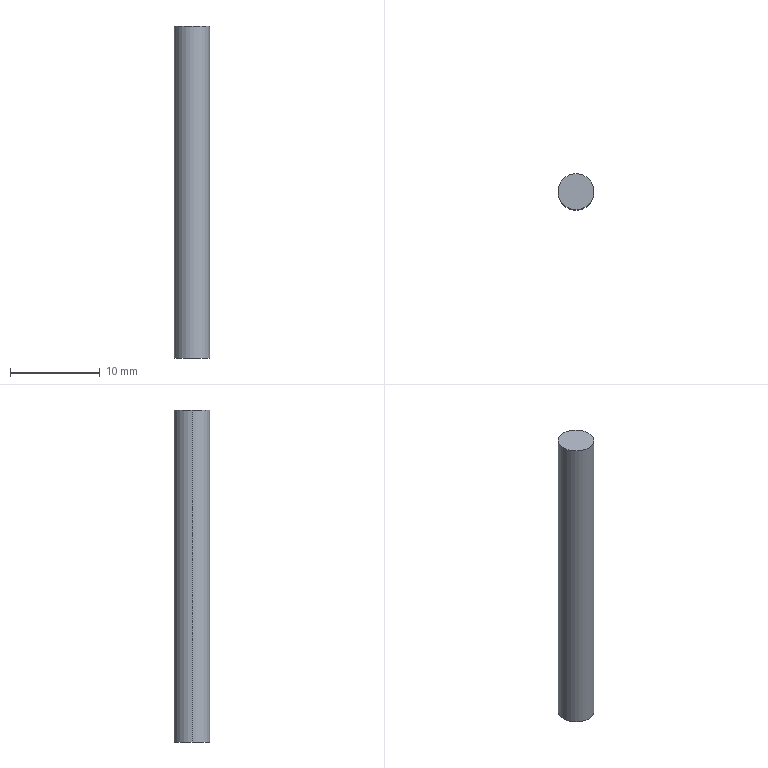Part | SolidWorks | features Extrusion 1 | 1 solid | 4 faces | box 4 x 4 x 37 mm | volume 464.956 mm3 | cylinder 2 | plane 2 | commonest cylinder face diameters 4 x2
STEP:
#1=CARTESIAN_POINT('',(2.,0.,37.));
#2=VERTEX_POINT('',#1);
#3=CARTESIAN_POINT('',(-2.,0.,37.));
#4=VERTEX_POINT('',#3);
#5=CARTESIAN_POINT('',(0.,0.,37.));
#6=DIRECTION('',(0.,0.,1.));
#7=DIRECTION('',(1.,0.,0.));
#8=AXIS2_PLACEMENT_3D('',#5,#6,#7);
#9=CIRCLE('',#8,2.);
#10=EDGE_CURVE('',#2,#4,#9,.T.);
#11=ORIENTED_EDGE('',*,*,#10,.F.);
#12=CARTESIAN_POINT('',(2.,0.,0.));
#13=VERTEX_POINT('',#12);
#14=CARTESIAN_POINT('',(2.,0.,37.));
#15=DIRECTION('',(0.,0.,-1.));
#16=VECTOR('',#15,1000.);
#17=LINE('',#14,#16);
#18=EDGE_CURVE('',#2,#13,#17,.T.);
#19=ORIENTED_EDGE('',*,*,#18,.T.);
#20=CARTESIAN_POINT('',(-2.,0.,0.));
#21=VERTEX_POINT('',#20);
#22=CARTESIAN_POINT('',(0.,0.,0.));
#23=DIRECTION('',(0.,0.,1.));
#24=DIRECTION('',(1.,0.,0.));
#25=AXIS2_PLACEMENT_3D('',#22,#23,#24);
#26=CIRCLE('',#25,2.);
#27=EDGE_CURVE('',#13,#21,#26,.T.);
#28=ORIENTED_EDGE('',*,*,#27,.T.);
#29=CARTESIAN_POINT('',(-2.,0.,37.));
#30=DIRECTION('',(0.,0.,-1.));
#31=VECTOR('',#30,1000.);
#32=LINE('',#29,#31);
#33=EDGE_CURVE('',#4,#21,#32,.T.);
#34=ORIENTED_EDGE('',*,*,#33,.F.);
#35=EDGE_LOOP('',(#11,#19,#28,#34));
#36=FACE_OUTER_BOUND('',#35,.T.);
#37=CARTESIAN_POINT('',(0.,0.,37.));
#38=DIRECTION('',(0.,0.,-1.));
#39=DIRECTION('',(-1.,0.,0.));
#40=AXIS2_PLACEMENT_3D('',#37,#38,#39);
#41=CYLINDRICAL_SURFACE('',#40,2.);
#42=ADVANCED_FACE('',(#36),#41,.T.);
#43=ORIENTED_EDGE('',*,*,#18,.F.);
#44=CARTESIAN_POINT('',(0.,0.,37.));
#45=DIRECTION('',(0.,0.,1.));
#46=DIRECTION('',(1.,0.,0.));
#47=AXIS2_PLACEMENT_3D('',#44,#45,#46);
#48=CIRCLE('',#47,2.);
#49=EDGE_CURVE('',#4,#2,#48,.T.);
#50=ORIENTED_EDGE('',*,*,#49,.F.);
#51=ORIENTED_EDGE('',*,*,#33,.T.);
#52=CARTESIAN_POINT('',(0.,0.,0.));
#53=DIRECTION('',(0.,0.,1.));
#54=DIRECTION('',(1.,0.,0.));
#55=AXIS2_PLACEMENT_3D('',#52,#53,#54);
#56=CIRCLE('',#55,2.);
#57=EDGE_CURVE('',#21,#13,#56,.T.);
#58=ORIENTED_EDGE('',*,*,#57,.T.);
#59=EDGE_LOOP('',(#43,#50,#51,#58));
#60=FACE_OUTER_BOUND('',#59,.T.);
#61=CARTESIAN_POINT('',(0.,0.,37.));
#62=DIRECTION('',(0.,0.,-1.));
#63=DIRECTION('',(-1.,0.,0.));
#64=AXIS2_PLACEMENT_3D('',#61,#62,#63);
#65=CYLINDRICAL_SURFACE('',#64,2.);
#66=ADVANCED_FACE('',(#60),#65,.T.);
#67=ORIENTED_EDGE('',*,*,#49,.T.);
#68=ORIENTED_EDGE('',*,*,#10,.T.);
#69=EDGE_LOOP('',(#67,#68));
#70=FACE_OUTER_BOUND('',#69,.T.);
#71=CARTESIAN_POINT('',(0.,0.,37.));
#72=DIRECTION('',(0.,0.,1.));
#73=DIRECTION('',(1.,0.,0.));
#74=AXIS2_PLACEMENT_3D('',#71,#72,#73);
#75=PLANE('',#74);
#76=ADVANCED_FACE('',(#70),#75,.T.);
#77=ORIENTED_EDGE('',*,*,#57,.F.);
#78=ORIENTED_EDGE('',*,*,#27,.F.);
#79=EDGE_LOOP('',(#77,#78));
#80=FACE_OUTER_BOUND('',#79,.T.);
#81=CARTESIAN_POINT('',(0.,0.,0.));
#82=DIRECTION('',(0.,0.,1.));
#83=DIRECTION('',(1.,0.,0.));
#84=AXIS2_PLACEMENT_3D('',#81,#82,#83);
#85=PLANE('',#84);
#86=ADVANCED_FACE('',(#80),#85,.F.);
#87=CLOSED_SHELL('',(#42,#66,#76,#86));
#88=MANIFOLD_SOLID_BREP('',#87);
#89=CARTESIAN_POINT('',(0.,0.,0.));
#90=DIRECTION('',(0.,0.,1.));
#91=DIRECTION('',(1.,0.,0.));
#92=AXIS2_PLACEMENT_3D('',#89,#90,#91);
#93=(LENGTH_UNIT()NAMED_UNIT(*)SI_UNIT(.MILLI.,.METRE.));
#94=UNCERTAINTY_MEASURE_WITH_UNIT(LENGTH_MEASURE(0.00001),#93,'','');
#95=(NAMED_UNIT(*)PLANE_ANGLE_UNIT()SI_UNIT($,.RADIAN.));
#96=(NAMED_UNIT(*)SI_UNIT($,.STERADIAN.)SOLID_ANGLE_UNIT());
#97=(GEOMETRIC_REPRESENTATION_CONTEXT(3)GLOBAL_UNCERTAINTY_ASSIGNED_CONTEXT((#94))GLOBAL_UNIT_ASSIGNED_CONTEXT((#93,#95,#96))REPRESENTATION_CONTEXT('',''));
#98=ADVANCED_BREP_SHAPE_REPRESENTATION('',(#88,#92),#97);